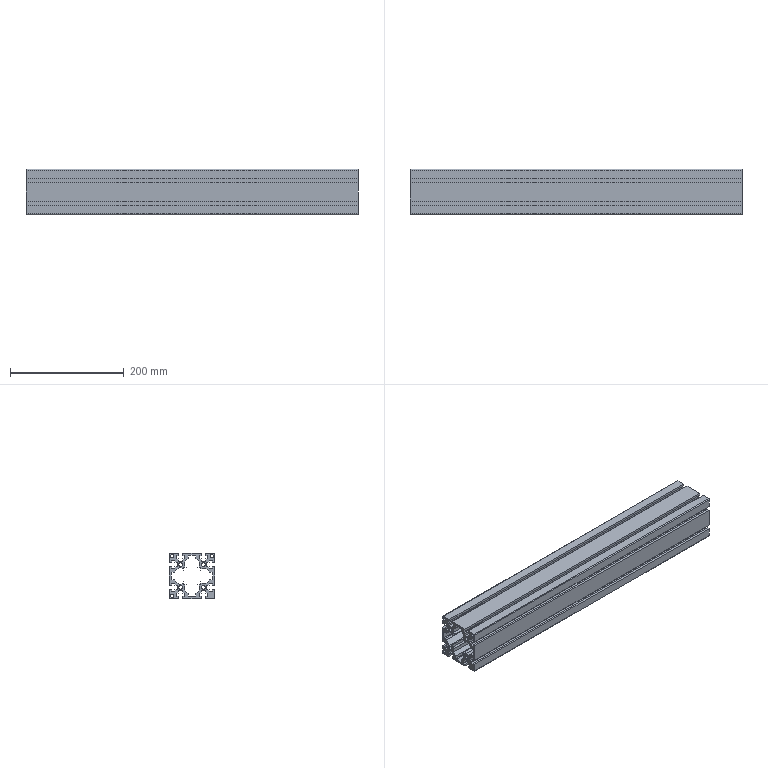Part | NX | 1 solid | 165 faces | box 585 x 80 x 80 mm | volume 1355618 mm3 | plane 146 | cylinder 19 | commonest cylinder face diameters 2 x8 3 x4 6.8 x4 6 x3